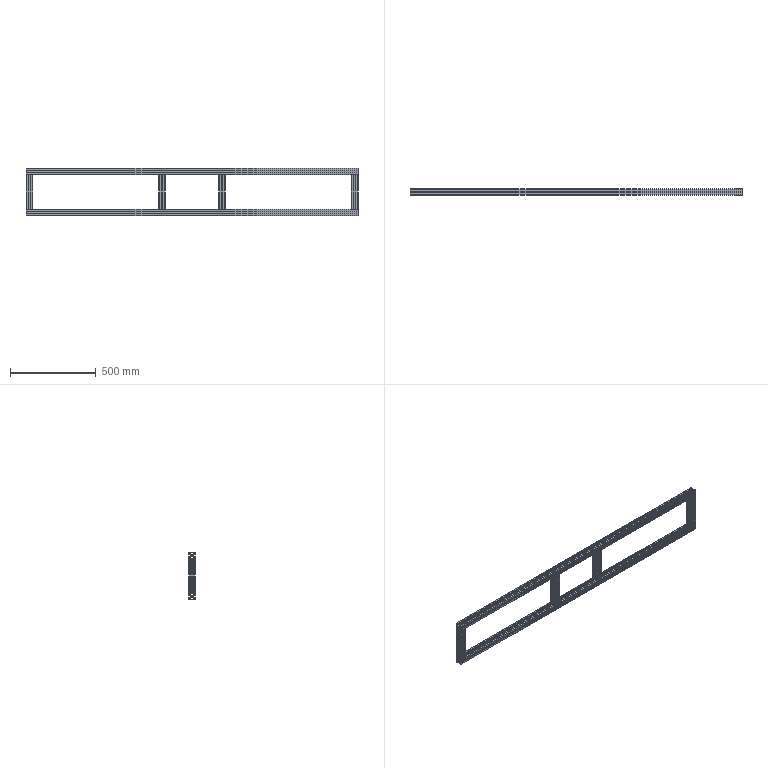Part | SolidWorks | features WeldMemberFeat 1, WeldmentFeature 1 | 6 solids | 552 faces | box 1940 x 40 x 280 mm | volume 2830666 mm3 | plane 468 | cylinder 84 | commonest cylinder face diameters 6 x48 9 x24 6.8 x12